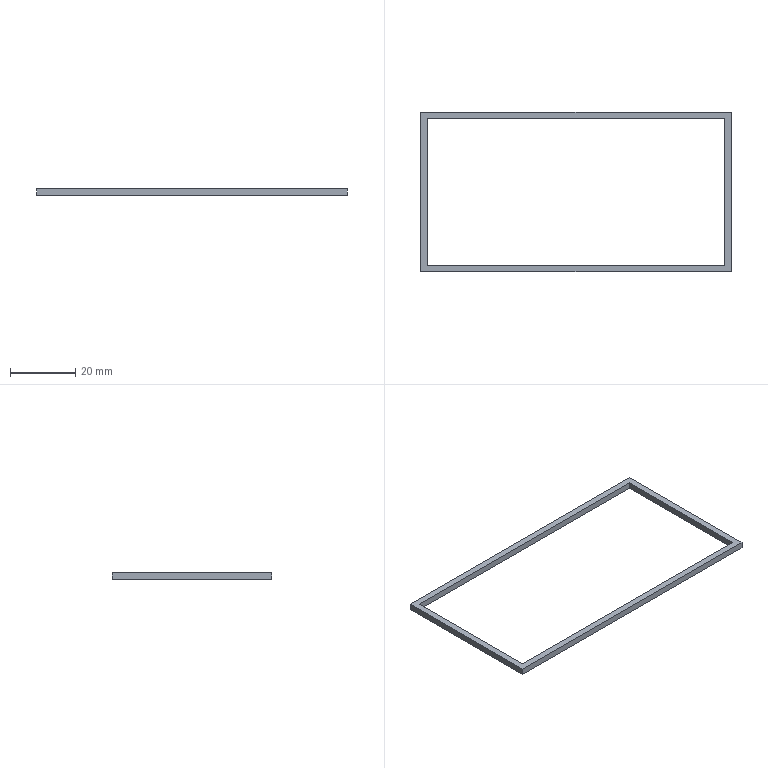Part | STEP file | K3HB_V_PACKING | 1 solid | 10 faces | box 95 x 48.8 x 2 mm | volume 1118 mm3 | plane 10
STEP:
#1=CARTESIAN_POINT('',(0.,0.,0.));
#2=DIRECTION('',(0.,0.,1.));
#3=DIRECTION('',(1.,0.,0.));
#4=AXIS2_PLACEMENT_3D('',#1,#2,#3);
#5=CARTESIAN_POINT('',(-47.5,24.4,2.));
#6=VERTEX_POINT('',#5);
#7=CARTESIAN_POINT('',(-47.5,-24.4,2.));
#8=VERTEX_POINT('',#7);
#9=CARTESIAN_POINT('',(-47.5,24.4,2.));
#10=DIRECTION('',(0.,-1.,0.));
#11=VECTOR('',#10,1.);
#12=LINE('',#9,#11);
#13=CARTESIAN_POINT('',(-47.5,-24.4,2.));
#14=DIRECTION('',(0.,0.,1.));
#15=DIRECTION('',(1.,0.,0.));
#16=AXIS2_PLACEMENT_3D('',#13,#14,#15);
#17=PLANE('',#16);
#18=CARTESIAN_POINT('',(0.,48.8));
#19=DIRECTION('',(0.,-1.));
#20=VECTOR('',#19,1.);
#21=LINE('',#18,#20);
#22=(GEOMETRIC_REPRESENTATION_CONTEXT(2)PARAMETRIC_REPRESENTATION_CONTEXT()REPRESENTATION_CONTEXT('',''));
#23=DEFINITIONAL_REPRESENTATION('',(#21),#22);
#24=PCURVE('',#17,#23);
#25=CARTESIAN_POINT('',(-47.5,24.4,2.));
#26=DIRECTION('',(1.,0.,0.));
#27=DIRECTION('',(0.,1.,0.));
#28=AXIS2_PLACEMENT_3D('',#25,#26,#27);
#29=PLANE('',#28);
#30=CARTESIAN_POINT('',(0.,0.));
#31=DIRECTION('',(-1.,0.));
#32=VECTOR('',#31,1.);
#33=LINE('',#30,#32);
#34=(GEOMETRIC_REPRESENTATION_CONTEXT(2)PARAMETRIC_REPRESENTATION_CONTEXT()REPRESENTATION_CONTEXT('',''));
#35=DEFINITIONAL_REPRESENTATION('',(#33),#34);
#36=PCURVE('',#29,#35);
#37=SURFACE_CURVE('',#12,(#24,#36),.PCURVE_S1.);
#38=EDGE_CURVE('',#6,#8,#37,.T.);
#39=ORIENTED_EDGE('',*,*,#38,.T.);
#40=CARTESIAN_POINT('',(47.5,-24.4,2.));
#41=VERTEX_POINT('',#40);
#42=CARTESIAN_POINT('',(-47.5,-24.4,2.));
#43=DIRECTION('',(1.,0.,0.));
#44=VECTOR('',#43,1.);
#45=LINE('',#42,#44);
#46=CARTESIAN_POINT('',(0.,0.));
#47=DIRECTION('',(1.,0.));
#48=VECTOR('',#47,1.);
#49=LINE('',#46,#48);
#50=(GEOMETRIC_REPRESENTATION_CONTEXT(2)PARAMETRIC_REPRESENTATION_CONTEXT()REPRESENTATION_CONTEXT('',''));
#51=DEFINITIONAL_REPRESENTATION('',(#49),#50);
#52=PCURVE('',#17,#51);
#53=CARTESIAN_POINT('',(-47.5,-24.4,2.));
#54=DIRECTION('',(0.,1.,0.));
#55=DIRECTION('',(0.,0.,1.));
#56=AXIS2_PLACEMENT_3D('',#53,#54,#55);
#57=PLANE('',#56);
#58=CARTESIAN_POINT('',(0.,0.));
#59=DIRECTION('',(0.,1.));
#60=VECTOR('',#59,1.);
#61=LINE('',#58,#60);
#62=(GEOMETRIC_REPRESENTATION_CONTEXT(2)PARAMETRIC_REPRESENTATION_CONTEXT()REPRESENTATION_CONTEXT('',''));
#63=DEFINITIONAL_REPRESENTATION('',(#61),#62);
#64=PCURVE('',#57,#63);
#65=SURFACE_CURVE('',#45,(#52,#64),.PCURVE_S1.);
#66=EDGE_CURVE('',#8,#41,#65,.T.);
#67=ORIENTED_EDGE('',*,*,#66,.T.);
#68=CARTESIAN_POINT('',(47.5,24.4,2.));
#69=VERTEX_POINT('',#68);
#70=CARTESIAN_POINT('',(47.5,24.4,2.));
#71=DIRECTION('',(0.,1.,0.));
#72=VECTOR('',#71,1.);
#73=LINE('',#70,#72);
#74=CARTESIAN_POINT('',(95.,48.8));
#75=DIRECTION('',(0.,1.));
#76=VECTOR('',#75,1.);
#77=LINE('',#74,#76);
#78=(GEOMETRIC_REPRESENTATION_CONTEXT(2)PARAMETRIC_REPRESENTATION_CONTEXT()REPRESENTATION_CONTEXT('',''));
#79=DEFINITIONAL_REPRESENTATION('',(#77),#78);
#80=PCURVE('',#17,#79);
#81=CARTESIAN_POINT('',(47.5,24.4,2.));
#82=DIRECTION('',(-1.,0.,0.));
#83=DIRECTION('',(0.,0.,1.));
#84=AXIS2_PLACEMENT_3D('',#81,#82,#83);
#85=PLANE('',#84);
#86=CARTESIAN_POINT('',(0.,0.));
#87=DIRECTION('',(0.,1.));
#88=VECTOR('',#87,1.);
#89=LINE('',#86,#88);
#90=(GEOMETRIC_REPRESENTATION_CONTEXT(2)PARAMETRIC_REPRESENTATION_CONTEXT()REPRESENTATION_CONTEXT('',''));
#91=DEFINITIONAL_REPRESENTATION('',(#89),#90);
#92=PCURVE('',#85,#91);
#93=SURFACE_CURVE('',#73,(#80,#92),.PCURVE_S1.);
#94=EDGE_CURVE('',#41,#69,#93,.T.);
#95=ORIENTED_EDGE('',*,*,#94,.T.);
#96=CARTESIAN_POINT('',(-47.5,24.4,2.));
#97=DIRECTION('',(-1.,0.,0.));
#98=VECTOR('',#97,1.);
#99=LINE('',#96,#98);
#100=CARTESIAN_POINT('',(0.,48.8));
#101=DIRECTION('',(-1.,0.));
#102=VECTOR('',#101,1.);
#103=LINE('',#100,#102);
#104=(GEOMETRIC_REPRESENTATION_CONTEXT(2)PARAMETRIC_REPRESENTATION_CONTEXT()REPRESENTATION_CONTEXT('',''));
#105=DEFINITIONAL_REPRESENTATION('',(#103),#104);
#106=PCURVE('',#17,#105);
#107=CARTESIAN_POINT('',(-47.5,24.4,2.));
#108=DIRECTION('',(0.,-1.,0.));
#109=DIRECTION('',(1.,0.,0.));
#110=AXIS2_PLACEMENT_3D('',#107,#108,#109);
#111=PLANE('',#110);
#112=CARTESIAN_POINT('',(0.,0.));
#113=DIRECTION('',(-1.,0.));
#114=VECTOR('',#113,1.);
#115=LINE('',#112,#114);
#116=(GEOMETRIC_REPRESENTATION_CONTEXT(2)PARAMETRIC_REPRESENTATION_CONTEXT()REPRESENTATION_CONTEXT('',''));
#117=DEFINITIONAL_REPRESENTATION('',(#115),#116);
#118=PCURVE('',#111,#117);
#119=SURFACE_CURVE('',#99,(#106,#118),.PCURVE_S1.);
#120=EDGE_CURVE('',#69,#6,#119,.T.);
#121=ORIENTED_EDGE('',*,*,#120,.T.);
#122=EDGE_LOOP('',(#39,#67,#95,#121));
#123=FACE_BOUND('',#122,.T.);
#124=CARTESIAN_POINT('',(-45.5,-22.4,2.));
#125=VERTEX_POINT('',#124);
#126=CARTESIAN_POINT('',(45.5,-22.4,2.));
#127=VERTEX_POINT('',#126);
#128=CARTESIAN_POINT('',(-45.5,-22.4,2.));
#129=DIRECTION('',(1.,0.,0.));
#130=VECTOR('',#129,1.);
#131=LINE('',#128,#130);
#132=CARTESIAN_POINT('',(2.,2.));
#133=DIRECTION('',(1.,0.));
#134=VECTOR('',#133,1.);
#135=LINE('',#132,#134);
#136=(GEOMETRIC_REPRESENTATION_CONTEXT(2)PARAMETRIC_REPRESENTATION_CONTEXT()REPRESENTATION_CONTEXT('',''));
#137=DEFINITIONAL_REPRESENTATION('',(#135),#136);
#138=PCURVE('',#17,#137);
#139=CARTESIAN_POINT('',(-45.5,-22.4,2.));
#140=DIRECTION('',(0.,1.,0.));
#141=DIRECTION('',(0.,0.,1.));
#142=AXIS2_PLACEMENT_3D('',#139,#140,#141);
#143=PLANE('',#142);
#144=CARTESIAN_POINT('',(0.,0.));
#145=DIRECTION('',(0.,1.));
#146=VECTOR('',#145,1.);
#147=LINE('',#144,#146);
#148=(GEOMETRIC_REPRESENTATION_CONTEXT(2)PARAMETRIC_REPRESENTATION_CONTEXT()REPRESENTATION_CONTEXT('',''));
#149=DEFINITIONAL_REPRESENTATION('',(#147),#148);
#150=PCURVE('',#143,#149);
#151=SURFACE_CURVE('',#131,(#138,#150),.PCURVE_S1.);
#152=EDGE_CURVE('',#125,#127,#151,.T.);
#153=ORIENTED_EDGE('',*,*,#152,.F.);
#154=CARTESIAN_POINT('',(-45.5,22.4,2.));
#155=VERTEX_POINT('',#154);
#156=CARTESIAN_POINT('',(-45.5,22.4,2.));
#157=DIRECTION('',(0.,-1.,0.));
#158=VECTOR('',#157,1.);
#159=LINE('',#156,#158);
#160=CARTESIAN_POINT('',(2.,46.8));
#161=DIRECTION('',(0.,-1.));
#162=VECTOR('',#161,1.);
#163=LINE('',#160,#162);
#164=(GEOMETRIC_REPRESENTATION_CONTEXT(2)PARAMETRIC_REPRESENTATION_CONTEXT()REPRESENTATION_CONTEXT('',''));
#165=DEFINITIONAL_REPRESENTATION('',(#163),#164);
#166=PCURVE('',#17,#165);
#167=CARTESIAN_POINT('',(-45.5,22.4,2.));
#168=DIRECTION('',(1.,0.,0.));
#169=DIRECTION('',(0.,1.,0.));
#170=AXIS2_PLACEMENT_3D('',#167,#168,#169);
#171=PLANE('',#170);
#172=CARTESIAN_POINT('',(0.,0.));
#173=DIRECTION('',(-1.,0.));
#174=VECTOR('',#173,1.);
#175=LINE('',#172,#174);
#176=(GEOMETRIC_REPRESENTATION_CONTEXT(2)PARAMETRIC_REPRESENTATION_CONTEXT()REPRESENTATION_CONTEXT('',''));
#177=DEFINITIONAL_REPRESENTATION('',(#175),#176);
#178=PCURVE('',#171,#177);
#179=SURFACE_CURVE('',#159,(#166,#178),.PCURVE_S1.);
#180=EDGE_CURVE('',#155,#125,#179,.T.);
#181=ORIENTED_EDGE('',*,*,#180,.F.);
#182=CARTESIAN_POINT('',(45.5,22.4,2.));
#183=VERTEX_POINT('',#182);
#184=CARTESIAN_POINT('',(-45.5,22.4,2.));
#185=DIRECTION('',(-1.,0.,0.));
#186=VECTOR('',#185,1.);
#187=LINE('',#184,#186);
#188=CARTESIAN_POINT('',(2.,46.8));
#189=DIRECTION('',(-1.,0.));
#190=VECTOR('',#189,1.);
#191=LINE('',#188,#190);
#192=(GEOMETRIC_REPRESENTATION_CONTEXT(2)PARAMETRIC_REPRESENTATION_CONTEXT()REPRESENTATION_CONTEXT('',''));
#193=DEFINITIONAL_REPRESENTATION('',(#191),#192);
#194=PCURVE('',#17,#193);
#195=CARTESIAN_POINT('',(-45.5,22.4,2.));
#196=DIRECTION('',(0.,-1.,0.));
#197=DIRECTION('',(1.,0.,0.));
#198=AXIS2_PLACEMENT_3D('',#195,#196,#197);
#199=PLANE('',#198);
#200=CARTESIAN_POINT('',(0.,0.));
#201=DIRECTION('',(-1.,0.));
#202=VECTOR('',#201,1.);
#203=LINE('',#200,#202);
#204=(GEOMETRIC_REPRESENTATION_CONTEXT(2)PARAMETRIC_REPRESENTATION_CONTEXT()REPRESENTATION_CONTEXT('',''));
#205=DEFINITIONAL_REPRESENTATION('',(#203),#204);
#206=PCURVE('',#199,#205);
#207=SURFACE_CURVE('',#187,(#194,#206),.PCURVE_S1.);
#208=EDGE_CURVE('',#183,#155,#207,.T.);
#209=ORIENTED_EDGE('',*,*,#208,.F.);
#210=CARTESIAN_POINT('',(45.5,22.4,2.));
#211=DIRECTION('',(0.,1.,0.));
#212=VECTOR('',#211,1.);
#213=LINE('',#210,#212);
#214=CARTESIAN_POINT('',(93.,46.8));
#215=DIRECTION('',(0.,1.));
#216=VECTOR('',#215,1.);
#217=LINE('',#214,#216);
#218=(GEOMETRIC_REPRESENTATION_CONTEXT(2)PARAMETRIC_REPRESENTATION_CONTEXT()REPRESENTATION_CONTEXT('',''));
#219=DEFINITIONAL_REPRESENTATION('',(#217),#218);
#220=PCURVE('',#17,#219);
#221=CARTESIAN_POINT('',(45.5,22.4,2.));
#222=DIRECTION('',(-1.,0.,0.));
#223=DIRECTION('',(0.,0.,1.));
#224=AXIS2_PLACEMENT_3D('',#221,#222,#223);
#225=PLANE('',#224);
#226=CARTESIAN_POINT('',(0.,0.));
#227=DIRECTION('',(0.,1.));
#228=VECTOR('',#227,1.);
#229=LINE('',#226,#228);
#230=(GEOMETRIC_REPRESENTATION_CONTEXT(2)PARAMETRIC_REPRESENTATION_CONTEXT()REPRESENTATION_CONTEXT('',''));
#231=DEFINITIONAL_REPRESENTATION('',(#229),#230);
#232=PCURVE('',#225,#231);
#233=SURFACE_CURVE('',#213,(#220,#232),.PCURVE_S1.);
#234=EDGE_CURVE('',#127,#183,#233,.T.);
#235=ORIENTED_EDGE('',*,*,#234,.F.);
#236=EDGE_LOOP('',(#153,#181,#209,#235));
#237=FACE_BOUND('',#236,.T.);
#238=ADVANCED_FACE('',(#123,#237),#17,.T.);
#239=CARTESIAN_POINT('',(-47.5,24.4,0.));
#240=VERTEX_POINT('',#239);
#241=CARTESIAN_POINT('',(-47.5,-24.4,0.));
#242=VERTEX_POINT('',#241);
#243=CARTESIAN_POINT('',(-47.5,24.4,0.));
#244=DIRECTION('',(0.,-1.,0.));
#245=VECTOR('',#244,1.);
#246=LINE('',#243,#245);
#247=CARTESIAN_POINT('',(-47.5,-24.4,0.));
#248=DIRECTION('',(0.,0.,1.));
#249=DIRECTION('',(1.,0.,0.));
#250=AXIS2_PLACEMENT_3D('',#247,#248,#249);
#251=PLANE('',#250);
#252=CARTESIAN_POINT('',(0.,48.8));
#253=DIRECTION('',(0.,-1.));
#254=VECTOR('',#253,1.);
#255=LINE('',#252,#254);
#256=(GEOMETRIC_REPRESENTATION_CONTEXT(2)PARAMETRIC_REPRESENTATION_CONTEXT()REPRESENTATION_CONTEXT('',''));
#257=DEFINITIONAL_REPRESENTATION('',(#255),#256);
#258=PCURVE('',#251,#257);
#259=CARTESIAN_POINT('',(0.,-2.));
#260=DIRECTION('',(-1.,0.));
#261=VECTOR('',#260,1.);
#262=LINE('',#259,#261);
#263=(GEOMETRIC_REPRESENTATION_CONTEXT(2)PARAMETRIC_REPRESENTATION_CONTEXT()REPRESENTATION_CONTEXT('',''));
#264=DEFINITIONAL_REPRESENTATION('',(#262),#263);
#265=PCURVE('',#29,#264);
#266=SURFACE_CURVE('',#246,(#258,#265),.PCURVE_S1.);
#267=EDGE_CURVE('',#240,#242,#266,.T.);
#268=ORIENTED_EDGE('',*,*,#267,.F.);
#269=CARTESIAN_POINT('',(47.5,24.4,0.));
#270=VERTEX_POINT('',#269);
#271=CARTESIAN_POINT('',(-47.5,24.4,0.));
#272=DIRECTION('',(-1.,0.,0.));
#273=VECTOR('',#272,1.);
#274=LINE('',#271,#273);
#275=CARTESIAN_POINT('',(0.,48.8));
#276=DIRECTION('',(-1.,0.));
#277=VECTOR('',#276,1.);
#278=LINE('',#275,#277);
#279=(GEOMETRIC_REPRESENTATION_CONTEXT(2)PARAMETRIC_REPRESENTATION_CONTEXT()REPRESENTATION_CONTEXT('',''));
#280=DEFINITIONAL_REPRESENTATION('',(#278),#279);
#281=PCURVE('',#251,#280);
#282=CARTESIAN_POINT('',(0.,-2.));
#283=DIRECTION('',(-1.,0.));
#284=VECTOR('',#283,1.);
#285=LINE('',#282,#284);
#286=(GEOMETRIC_REPRESENTATION_CONTEXT(2)PARAMETRIC_REPRESENTATION_CONTEXT()REPRESENTATION_CONTEXT('',''));
#287=DEFINITIONAL_REPRESENTATION('',(#285),#286);
#288=PCURVE('',#111,#287);
#289=SURFACE_CURVE('',#274,(#281,#288),.PCURVE_S1.);
#290=EDGE_CURVE('',#270,#240,#289,.T.);
#291=ORIENTED_EDGE('',*,*,#290,.F.);
#292=CARTESIAN_POINT('',(47.5,-24.4,0.));
#293=VERTEX_POINT('',#292);
#294=CARTESIAN_POINT('',(47.5,24.4,0.));
#295=DIRECTION('',(0.,1.,0.));
#296=VECTOR('',#295,1.);
#297=LINE('',#294,#296);
#298=CARTESIAN_POINT('',(95.,48.8));
#299=DIRECTION('',(0.,1.));
#300=VECTOR('',#299,1.);
#301=LINE('',#298,#300);
#302=(GEOMETRIC_REPRESENTATION_CONTEXT(2)PARAMETRIC_REPRESENTATION_CONTEXT()REPRESENTATION_CONTEXT('',''));
#303=DEFINITIONAL_REPRESENTATION('',(#301),#302);
#304=PCURVE('',#251,#303);
#305=CARTESIAN_POINT('',(-2.,0.));
#306=DIRECTION('',(0.,1.));
#307=VECTOR('',#306,1.);
#308=LINE('',#305,#307);
#309=(GEOMETRIC_REPRESENTATION_CONTEXT(2)PARAMETRIC_REPRESENTATION_CONTEXT()REPRESENTATION_CONTEXT('',''));
#310=DEFINITIONAL_REPRESENTATION('',(#308),#309);
#311=PCURVE('',#85,#310);
#312=SURFACE_CURVE('',#297,(#304,#311),.PCURVE_S1.);
#313=EDGE_CURVE('',#293,#270,#312,.T.);
#314=ORIENTED_EDGE('',*,*,#313,.F.);
#315=CARTESIAN_POINT('',(-47.5,-24.4,0.));
#316=DIRECTION('',(1.,0.,0.));
#317=VECTOR('',#316,1.);
#318=LINE('',#315,#317);
#319=CARTESIAN_POINT('',(0.,0.));
#320=DIRECTION('',(1.,0.));
#321=VECTOR('',#320,1.);
#322=LINE('',#319,#321);
#323=(GEOMETRIC_REPRESENTATION_CONTEXT(2)PARAMETRIC_REPRESENTATION_CONTEXT()REPRESENTATION_CONTEXT('',''));
#324=DEFINITIONAL_REPRESENTATION('',(#322),#323);
#325=PCURVE('',#251,#324);
#326=CARTESIAN_POINT('',(-2.,0.));
#327=DIRECTION('',(0.,1.));
#328=VECTOR('',#327,1.);
#329=LINE('',#326,#328);
#330=(GEOMETRIC_REPRESENTATION_CONTEXT(2)PARAMETRIC_REPRESENTATION_CONTEXT()REPRESENTATION_CONTEXT('',''));
#331=DEFINITIONAL_REPRESENTATION('',(#329),#330);
#332=PCURVE('',#57,#331);
#333=SURFACE_CURVE('',#318,(#325,#332),.PCURVE_S1.);
#334=EDGE_CURVE('',#242,#293,#333,.T.);
#335=ORIENTED_EDGE('',*,*,#334,.F.);
#336=EDGE_LOOP('',(#268,#291,#314,#335));
#337=FACE_BOUND('',#336,.T.);
#338=CARTESIAN_POINT('',(-45.5,22.4,0.));
#339=VERTEX_POINT('',#338);
#340=CARTESIAN_POINT('',(-45.5,-22.4,0.));
#341=VERTEX_POINT('',#340);
#342=CARTESIAN_POINT('',(-45.5,22.4,0.));
#343=DIRECTION('',(0.,-1.,0.));
#344=VECTOR('',#343,1.);
#345=LINE('',#342,#344);
#346=CARTESIAN_POINT('',(2.,46.8));
#347=DIRECTION('',(0.,-1.));
#348=VECTOR('',#347,1.);
#349=LINE('',#346,#348);
#350=(GEOMETRIC_REPRESENTATION_CONTEXT(2)PARAMETRIC_REPRESENTATION_CONTEXT()REPRESENTATION_CONTEXT('',''));
#351=DEFINITIONAL_REPRESENTATION('',(#349),#350);
#352=PCURVE('',#251,#351);
#353=CARTESIAN_POINT('',(0.,-2.));
#354=DIRECTION('',(-1.,0.));
#355=VECTOR('',#354,1.);
#356=LINE('',#353,#355);
#357=(GEOMETRIC_REPRESENTATION_CONTEXT(2)PARAMETRIC_REPRESENTATION_CONTEXT()REPRESENTATION_CONTEXT('',''));
#358=DEFINITIONAL_REPRESENTATION('',(#356),#357);
#359=PCURVE('',#171,#358);
#360=SURFACE_CURVE('',#345,(#352,#359),.PCURVE_S1.);
#361=EDGE_CURVE('',#339,#341,#360,.T.);
#362=ORIENTED_EDGE('',*,*,#361,.T.);
#363=CARTESIAN_POINT('',(45.5,-22.4,0.));
#364=VERTEX_POINT('',#363);
#365=CARTESIAN_POINT('',(-45.5,-22.4,0.));
#366=DIRECTION('',(1.,0.,0.));
#367=VECTOR('',#366,1.);
#368=LINE('',#365,#367);
#369=CARTESIAN_POINT('',(2.,2.));
#370=DIRECTION('',(1.,0.));
#371=VECTOR('',#370,1.);
#372=LINE('',#369,#371);
#373=(GEOMETRIC_REPRESENTATION_CONTEXT(2)PARAMETRIC_REPRESENTATION_CONTEXT()REPRESENTATION_CONTEXT('',''));
#374=DEFINITIONAL_REPRESENTATION('',(#372),#373);
#375=PCURVE('',#251,#374);
#376=CARTESIAN_POINT('',(-2.,0.));
#377=DIRECTION('',(0.,1.));
#378=VECTOR('',#377,1.);
#379=LINE('',#376,#378);
#380=(GEOMETRIC_REPRESENTATION_CONTEXT(2)PARAMETRIC_REPRESENTATION_CONTEXT()REPRESENTATION_CONTEXT('',''));
#381=DEFINITIONAL_REPRESENTATION('',(#379),#380);
#382=PCURVE('',#143,#381);
#383=SURFACE_CURVE('',#368,(#375,#382),.PCURVE_S1.);
#384=EDGE_CURVE('',#341,#364,#383,.T.);
#385=ORIENTED_EDGE('',*,*,#384,.T.);
#386=CARTESIAN_POINT('',(45.5,22.4,0.));
#387=VERTEX_POINT('',#386);
#388=CARTESIAN_POINT('',(45.5,22.4,0.));
#389=DIRECTION('',(0.,1.,0.));
#390=VECTOR('',#389,1.);
#391=LINE('',#388,#390);
#392=CARTESIAN_POINT('',(93.,46.8));
#393=DIRECTION('',(0.,1.));
#394=VECTOR('',#393,1.);
#395=LINE('',#392,#394);
#396=(GEOMETRIC_REPRESENTATION_CONTEXT(2)PARAMETRIC_REPRESENTATION_CONTEXT()REPRESENTATION_CONTEXT('',''));
#397=DEFINITIONAL_REPRESENTATION('',(#395),#396);
#398=PCURVE('',#251,#397);
#399=CARTESIAN_POINT('',(-2.,0.));
#400=DIRECTION('',(0.,1.));
#401=VECTOR('',#400,1.);
#402=LINE('',#399,#401);
#403=(GEOMETRIC_REPRESENTATION_CONTEXT(2)PARAMETRIC_REPRESENTATION_CONTEXT()REPRESENTATION_CONTEXT('',''));
#404=DEFINITIONAL_REPRESENTATION('',(#402),#403);
#405=PCURVE('',#225,#404);
#406=SURFACE_CURVE('',#391,(#398,#405),.PCURVE_S1.);
#407=EDGE_CURVE('',#364,#387,#406,.T.);
#408=ORIENTED_EDGE('',*,*,#407,.T.);
#409=CARTESIAN_POINT('',(-45.5,22.4,0.));
#410=DIRECTION('',(-1.,0.,0.));
#411=VECTOR('',#410,1.);
#412=LINE('',#409,#411);
#413=CARTESIAN_POINT('',(2.,46.8));
#414=DIRECTION('',(-1.,0.));
#415=VECTOR('',#414,1.);
#416=LINE('',#413,#415);
#417=(GEOMETRIC_REPRESENTATION_CONTEXT(2)PARAMETRIC_REPRESENTATION_CONTEXT()REPRESENTATION_CONTEXT('',''));
#418=DEFINITIONAL_REPRESENTATION('',(#416),#417);
#419=PCURVE('',#251,#418);
#420=CARTESIAN_POINT('',(0.,-2.));
#421=DIRECTION('',(-1.,0.));
#422=VECTOR('',#421,1.);
#423=LINE('',#420,#422);
#424=(GEOMETRIC_REPRESENTATION_CONTEXT(2)PARAMETRIC_REPRESENTATION_CONTEXT()REPRESENTATION_CONTEXT('',''));
#425=DEFINITIONAL_REPRESENTATION('',(#423),#424);
#426=PCURVE('',#199,#425);
#427=SURFACE_CURVE('',#412,(#419,#426),.PCURVE_S1.);
#428=EDGE_CURVE('',#387,#339,#427,.T.);
#429=ORIENTED_EDGE('',*,*,#428,.T.);
#430=EDGE_LOOP('',(#362,#385,#408,#429));
#431=FACE_BOUND('',#430,.T.);
#432=ADVANCED_FACE('',(#337,#431),#251,.F.);
#433=ORIENTED_EDGE('',*,*,#267,.T.);
#434=CARTESIAN_POINT('',(-47.5,-24.4,2.));
#435=DIRECTION('',(0.,0.,-1.));
#436=VECTOR('',#435,1.);
#437=LINE('',#434,#436);
#438=CARTESIAN_POINT('',(-48.8,0.));
#439=DIRECTION('',(0.,-1.));
#440=VECTOR('',#439,1.);
#441=LINE('',#438,#440);
#442=(GEOMETRIC_REPRESENTATION_CONTEXT(2)PARAMETRIC_REPRESENTATION_CONTEXT()REPRESENTATION_CONTEXT('',''));
#443=DEFINITIONAL_REPRESENTATION('',(#441),#442);
#444=PCURVE('',#29,#443);
#445=CARTESIAN_POINT('',(0.,0.));
#446=DIRECTION('',(-1.,0.));
#447=VECTOR('',#446,1.);
#448=LINE('',#445,#447);
#449=(GEOMETRIC_REPRESENTATION_CONTEXT(2)PARAMETRIC_REPRESENTATION_CONTEXT()REPRESENTATION_CONTEXT('',''));
#450=DEFINITIONAL_REPRESENTATION('',(#448),#449);
#451=PCURVE('',#57,#450);
#452=SURFACE_CURVE('',#437,(#444,#451),.PCURVE_S1.);
#453=EDGE_CURVE('',#8,#242,#452,.T.);
#454=ORIENTED_EDGE('',*,*,#453,.F.);
#455=ORIENTED_EDGE('',*,*,#38,.F.);
#456=CARTESIAN_POINT('',(-47.5,24.4,2.));
#457=DIRECTION('',(0.,0.,-1.));
#458=VECTOR('',#457,1.);
#459=LINE('',#456,#458);
#460=CARTESIAN_POINT('',(0.,0.));
#461=DIRECTION('',(0.,-1.));
#462=VECTOR('',#461,1.);
#463=LINE('',#460,#462);
#464=(GEOMETRIC_REPRESENTATION_CONTEXT(2)PARAMETRIC_REPRESENTATION_CONTEXT()REPRESENTATION_CONTEXT('',''));
#465=DEFINITIONAL_REPRESENTATION('',(#463),#464);
#466=PCURVE('',#29,#465);
#467=CARTESIAN_POINT('',(0.,0.));
#468=DIRECTION('',(0.,-1.));
#469=VECTOR('',#468,1.);
#470=LINE('',#467,#469);
#471=(GEOMETRIC_REPRESENTATION_CONTEXT(2)PARAMETRIC_REPRESENTATION_CONTEXT()REPRESENTATION_CONTEXT('',''));
#472=DEFINITIONAL_REPRESENTATION('',(#470),#471);
#473=PCURVE('',#111,#472);
#474=SURFACE_CURVE('',#459,(#466,#473),.PCURVE_S1.);
#475=EDGE_CURVE('',#6,#240,#474,.T.);
#476=ORIENTED_EDGE('',*,*,#475,.T.);
#477=EDGE_LOOP('',(#433,#454,#455,#476));
#478=FACE_BOUND('',#477,.T.);
#479=ADVANCED_FACE('',(#478),#29,.F.);
#480=ORIENTED_EDGE('',*,*,#334,.T.);
#481=CARTESIAN_POINT('',(47.5,-24.4,2.));
#482=DIRECTION('',(0.,0.,-1.));
#483=VECTOR('',#482,1.);
#484=LINE('',#481,#483);
#485=CARTESIAN_POINT('',(0.,95.));
#486=DIRECTION('',(-1.,0.));
#487=VECTOR('',#486,1.);
#488=LINE('',#485,#487);
#489=(GEOMETRIC_REPRESENTATION_CONTEXT(2)PARAMETRIC_REPRESENTATION_CONTEXT()REPRESENTATION_CONTEXT('',''));
#490=DEFINITIONAL_REPRESENTATION('',(#488),#489);
#491=PCURVE('',#57,#490);
#492=CARTESIAN_POINT('',(0.,-48.8));
#493=DIRECTION('',(-1.,0.));
#494=VECTOR('',#493,1.);
#495=LINE('',#492,#494);
#496=(GEOMETRIC_REPRESENTATION_CONTEXT(2)PARAMETRIC_REPRESENTATION_CONTEXT()REPRESENTATION_CONTEXT('',''));
#497=DEFINITIONAL_REPRESENTATION('',(#495),#496);
#498=PCURVE('',#85,#497);
#499=SURFACE_CURVE('',#484,(#491,#498),.PCURVE_S1.);
#500=EDGE_CURVE('',#41,#293,#499,.T.);
#501=ORIENTED_EDGE('',*,*,#500,.F.);
#502=ORIENTED_EDGE('',*,*,#66,.F.);
#503=ORIENTED_EDGE('',*,*,#453,.T.);
#504=EDGE_LOOP('',(#480,#501,#502,#503));
#505=FACE_BOUND('',#504,.T.);
#506=ADVANCED_FACE('',(#505),#57,.F.);
#507=ORIENTED_EDGE('',*,*,#313,.T.);
#508=CARTESIAN_POINT('',(47.5,24.4,2.));
#509=DIRECTION('',(0.,0.,-1.));
#510=VECTOR('',#509,1.);
#511=LINE('',#508,#510);
#512=CARTESIAN_POINT('',(0.,0.));
#513=DIRECTION('',(-1.,0.));
#514=VECTOR('',#513,1.);
#515=LINE('',#512,#514);
#516=(GEOMETRIC_REPRESENTATION_CONTEXT(2)PARAMETRIC_REPRESENTATION_CONTEXT()REPRESENTATION_CONTEXT('',''));
#517=DEFINITIONAL_REPRESENTATION('',(#515),#516);
#518=PCURVE('',#85,#517);
#519=CARTESIAN_POINT('',(95.,0.));
#520=DIRECTION('',(0.,-1.));
#521=VECTOR('',#520,1.);
#522=LINE('',#519,#521);
#523=(GEOMETRIC_REPRESENTATION_CONTEXT(2)PARAMETRIC_REPRESENTATION_CONTEXT()REPRESENTATION_CONTEXT('',''));
#524=DEFINITIONAL_REPRESENTATION('',(#522),#523);
#525=PCURVE('',#111,#524);
#526=SURFACE_CURVE('',#511,(#518,#525),.PCURVE_S1.);
#527=EDGE_CURVE('',#69,#270,#526,.T.);
#528=ORIENTED_EDGE('',*,*,#527,.F.);
#529=ORIENTED_EDGE('',*,*,#94,.F.);
#530=ORIENTED_EDGE('',*,*,#500,.T.);
#531=EDGE_LOOP('',(#507,#528,#529,#530));
#532=FACE_BOUND('',#531,.T.);
#533=ADVANCED_FACE('',(#532),#85,.F.);
#534=ORIENTED_EDGE('',*,*,#290,.T.);
#535=ORIENTED_EDGE('',*,*,#475,.F.);
#536=ORIENTED_EDGE('',*,*,#120,.F.);
#537=ORIENTED_EDGE('',*,*,#527,.T.);
#538=EDGE_LOOP('',(#534,#535,#536,#537));
#539=FACE_BOUND('',#538,.T.);
#540=ADVANCED_FACE('',(#539),#111,.F.);
#541=ORIENTED_EDGE('',*,*,#361,.F.);
#542=CARTESIAN_POINT('',(-45.5,22.4,2.));
#543=DIRECTION('',(0.,0.,-1.));
#544=VECTOR('',#543,1.);
#545=LINE('',#542,#544);
#546=CARTESIAN_POINT('',(0.,0.));
#547=DIRECTION('',(0.,-1.));
#548=VECTOR('',#547,1.);
#549=LINE('',#546,#548);
#550=(GEOMETRIC_REPRESENTATION_CONTEXT(2)PARAMETRIC_REPRESENTATION_CONTEXT()REPRESENTATION_CONTEXT('',''));
#551=DEFINITIONAL_REPRESENTATION('',(#549),#550);
#552=PCURVE('',#171,#551);
#553=CARTESIAN_POINT('',(0.,0.));
#554=DIRECTION('',(0.,-1.));
#555=VECTOR('',#554,1.);
#556=LINE('',#553,#555);
#557=(GEOMETRIC_REPRESENTATION_CONTEXT(2)PARAMETRIC_REPRESENTATION_CONTEXT()REPRESENTATION_CONTEXT('',''));
#558=DEFINITIONAL_REPRESENTATION('',(#556),#557);
#559=PCURVE('',#199,#558);
#560=SURFACE_CURVE('',#545,(#552,#559),.PCURVE_S1.);
#561=EDGE_CURVE('',#155,#339,#560,.T.);
#562=ORIENTED_EDGE('',*,*,#561,.F.);
#563=ORIENTED_EDGE('',*,*,#180,.T.);
#564=CARTESIAN_POINT('',(-45.5,-22.4,2.));
#565=DIRECTION('',(0.,0.,-1.));
#566=VECTOR('',#565,1.);
#567=LINE('',#564,#566);
#568=CARTESIAN_POINT('',(-44.8,0.));
#569=DIRECTION('',(0.,-1.));
#570=VECTOR('',#569,1.);
#571=LINE('',#568,#570);
#572=(GEOMETRIC_REPRESENTATION_CONTEXT(2)PARAMETRIC_REPRESENTATION_CONTEXT()REPRESENTATION_CONTEXT('',''));
#573=DEFINITIONAL_REPRESENTATION('',(#571),#572);
#574=PCURVE('',#171,#573);
#575=CARTESIAN_POINT('',(0.,0.));
#576=DIRECTION('',(-1.,0.));
#577=VECTOR('',#576,1.);
#578=LINE('',#575,#577);
#579=(GEOMETRIC_REPRESENTATION_CONTEXT(2)PARAMETRIC_REPRESENTATION_CONTEXT()REPRESENTATION_CONTEXT('',''));
#580=DEFINITIONAL_REPRESENTATION('',(#578),#579);
#581=PCURVE('',#143,#580);
#582=SURFACE_CURVE('',#567,(#574,#581),.PCURVE_S1.);
#583=EDGE_CURVE('',#125,#341,#582,.T.);
#584=ORIENTED_EDGE('',*,*,#583,.T.);
#585=EDGE_LOOP('',(#541,#562,#563,#584));
#586=FACE_BOUND('',#585,.T.);
#587=ADVANCED_FACE('',(#586),#171,.T.);
#588=ORIENTED_EDGE('',*,*,#384,.F.);
#589=ORIENTED_EDGE('',*,*,#583,.F.);
#590=ORIENTED_EDGE('',*,*,#152,.T.);
#591=CARTESIAN_POINT('',(45.5,-22.4,2.));
#592=DIRECTION('',(0.,0.,-1.));
#593=VECTOR('',#592,1.);
#594=LINE('',#591,#593);
#595=CARTESIAN_POINT('',(0.,91.));
#596=DIRECTION('',(-1.,0.));
#597=VECTOR('',#596,1.);
#598=LINE('',#595,#597);
#599=(GEOMETRIC_REPRESENTATION_CONTEXT(2)PARAMETRIC_REPRESENTATION_CONTEXT()REPRESENTATION_CONTEXT('',''));
#600=DEFINITIONAL_REPRESENTATION('',(#598),#599);
#601=PCURVE('',#143,#600);
#602=CARTESIAN_POINT('',(0.,-44.8));
#603=DIRECTION('',(-1.,0.));
#604=VECTOR('',#603,1.);
#605=LINE('',#602,#604);
#606=(GEOMETRIC_REPRESENTATION_CONTEXT(2)PARAMETRIC_REPRESENTATION_CONTEXT()REPRESENTATION_CONTEXT('',''));
#607=DEFINITIONAL_REPRESENTATION('',(#605),#606);
#608=PCURVE('',#225,#607);
#609=SURFACE_CURVE('',#594,(#601,#608),.PCURVE_S1.);
#610=EDGE_CURVE('',#127,#364,#609,.T.);
#611=ORIENTED_EDGE('',*,*,#610,.T.);
#612=EDGE_LOOP('',(#588,#589,#590,#611));
#613=FACE_BOUND('',#612,.T.);
#614=ADVANCED_FACE('',(#613),#143,.T.);
#615=ORIENTED_EDGE('',*,*,#407,.F.);
#616=ORIENTED_EDGE('',*,*,#610,.F.);
#617=ORIENTED_EDGE('',*,*,#234,.T.);
#618=CARTESIAN_POINT('',(45.5,22.4,2.));
#619=DIRECTION('',(0.,0.,-1.));
#620=VECTOR('',#619,1.);
#621=LINE('',#618,#620);
#622=CARTESIAN_POINT('',(0.,0.));
#623=DIRECTION('',(-1.,0.));
#624=VECTOR('',#623,1.);
#625=LINE('',#622,#624);
#626=(GEOMETRIC_REPRESENTATION_CONTEXT(2)PARAMETRIC_REPRESENTATION_CONTEXT()REPRESENTATION_CONTEXT('',''));
#627=DEFINITIONAL_REPRESENTATION('',(#625),#626);
#628=PCURVE('',#225,#627);
#629=CARTESIAN_POINT('',(91.,0.));
#630=DIRECTION('',(0.,-1.));
#631=VECTOR('',#630,1.);
#632=LINE('',#629,#631);
#633=(GEOMETRIC_REPRESENTATION_CONTEXT(2)PARAMETRIC_REPRESENTATION_CONTEXT()REPRESENTATION_CONTEXT('',''));
#634=DEFINITIONAL_REPRESENTATION('',(#632),#633);
#635=PCURVE('',#199,#634);
#636=SURFACE_CURVE('',#621,(#628,#635),.PCURVE_S1.);
#637=EDGE_CURVE('',#183,#387,#636,.T.);
#638=ORIENTED_EDGE('',*,*,#637,.T.);
#639=EDGE_LOOP('',(#615,#616,#617,#638));
#640=FACE_BOUND('',#639,.T.);
#641=ADVANCED_FACE('',(#640),#225,.T.);
#642=ORIENTED_EDGE('',*,*,#428,.F.);
#643=ORIENTED_EDGE('',*,*,#637,.F.);
#644=ORIENTED_EDGE('',*,*,#208,.T.);
#645=ORIENTED_EDGE('',*,*,#561,.T.);
#646=EDGE_LOOP('',(#642,#643,#644,#645));
#647=FACE_BOUND('',#646,.T.);
#648=ADVANCED_FACE('',(#647),#199,.T.);
#649=CLOSED_SHELL('',(#238,#432,#479,#506,#533,#540,#587,#614,#641,#648));
#650=MANIFOLD_SOLID_BREP('',#649);
#651=(LENGTH_UNIT()NAMED_UNIT(*)SI_UNIT(.MILLI.,.METRE.));
#652=UNCERTAINTY_MEASURE_WITH_UNIT(LENGTH_MEASURE(0.0000001),#651,'','');
#653=(NAMED_UNIT(*)PLANE_ANGLE_UNIT()SI_UNIT($,.RADIAN.));
#654=(NAMED_UNIT(*)SI_UNIT($,.STERADIAN.)SOLID_ANGLE_UNIT());
#655=(GEOMETRIC_REPRESENTATION_CONTEXT(3)GLOBAL_UNCERTAINTY_ASSIGNED_CONTEXT((#652))GLOBAL_UNIT_ASSIGNED_CONTEXT((#651,#653,#654))REPRESENTATION_CONTEXT('',''));
#656=ADVANCED_BREP_SHAPE_REPRESENTATION('',(#4,#650),#655);